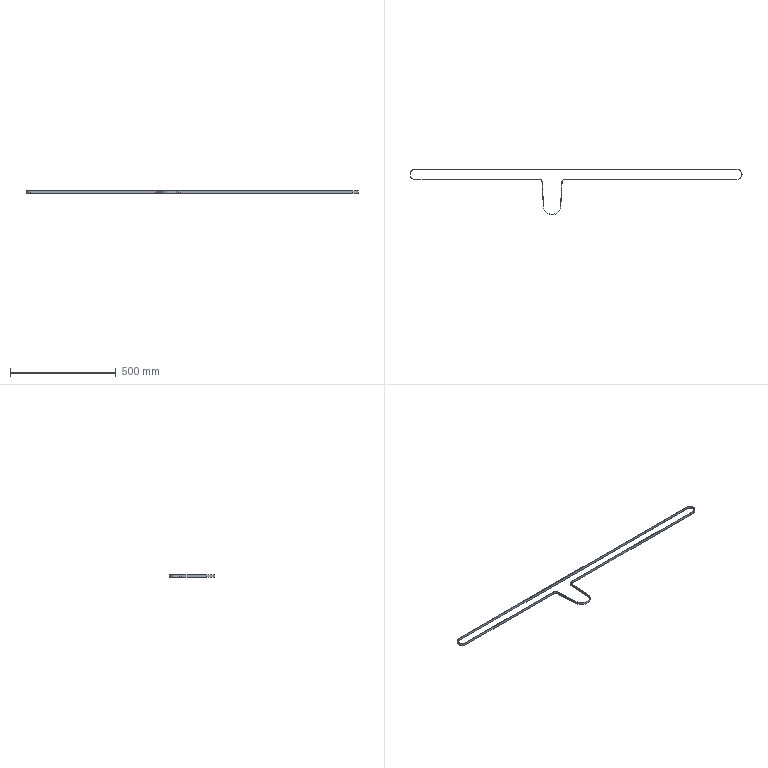Part | NX | features BREP 1 | 1 solid | 24 faces | box 1568 x 214.1 x 12 mm | volume 49856 mm3 | cylinder 12 | plane 12 | commonest cylinder face diameters 45 x3 47.4 x3 25 x2 27.4 x2 80 x1 82.4 x1
STEP:
#1=CARTESIAN_POINT('',(1415.214,8.857,-2.25));
#2=VERTEX_POINT('',#1);
#3=CARTESIAN_POINT('',(1392.714,31.357,-2.25));
#4=VERTEX_POINT('',#3);
#5=CARTESIAN_POINT('',(1392.714,8.857,-2.25));
#6=DIRECTION('',(0.,0.,1.));
#7=DIRECTION('',(-1.,0.,0.));
#8=AXIS2_PLACEMENT_3D('',#5,#6,#7);
#9=CIRCLE('',#8,22.5);
#10=EDGE_CURVE('',#2,#4,#9,.T.);
#11=ORIENTED_EDGE('',*,*,#10,.F.);
#12=CARTESIAN_POINT('',(1415.214,8.857,9.75));
#13=VERTEX_POINT('',#12);
#14=CARTESIAN_POINT('',(1415.214,8.857,-2.25));
#15=DIRECTION('',(0.,0.,1.));
#16=VECTOR('',#15,1000.);
#17=LINE('',#14,#16);
#18=EDGE_CURVE('',#2,#13,#17,.T.);
#19=ORIENTED_EDGE('',*,*,#18,.T.);
#20=CARTESIAN_POINT('',(1392.714,31.357,9.75));
#21=VERTEX_POINT('',#20);
#22=CARTESIAN_POINT('',(1392.714,8.857,9.75));
#23=DIRECTION('',(0.,0.,1.));
#24=DIRECTION('',(-1.,0.,0.));
#25=AXIS2_PLACEMENT_3D('',#22,#23,#24);
#26=CIRCLE('',#25,22.5);
#27=EDGE_CURVE('',#13,#21,#26,.T.);
#28=ORIENTED_EDGE('',*,*,#27,.T.);
#29=CARTESIAN_POINT('',(1392.714,31.357,-2.25));
#30=DIRECTION('',(0.,0.,1.));
#31=VECTOR('',#30,1000.);
#32=LINE('',#29,#31);
#33=EDGE_CURVE('',#4,#21,#32,.T.);
#34=ORIENTED_EDGE('',*,*,#33,.F.);
#35=EDGE_LOOP('',(#11,#19,#28,#34));
#36=FACE_BOUND('',#35,.T.);
#37=CARTESIAN_POINT('',(1392.714,8.857,-2.25));
#38=DIRECTION('',(0.,0.,1.));
#39=DIRECTION('',(1.,0.,0.));
#40=AXIS2_PLACEMENT_3D('',#37,#38,#39);
#41=CYLINDRICAL_SURFACE('',#40,22.5);
#42=ADVANCED_FACE('',(#36),#41,.F.);
#43=CARTESIAN_POINT('',(1392.714,-14.843,-2.25));
#44=VERTEX_POINT('',#43);
#45=CARTESIAN_POINT('',(1416.414,8.857,-2.25));
#46=VERTEX_POINT('',#45);
#47=CARTESIAN_POINT('',(1392.714,8.857,-2.25));
#48=DIRECTION('',(0.,0.,1.));
#49=DIRECTION('',(1.,0.,0.));
#50=AXIS2_PLACEMENT_3D('',#47,#48,#49);
#51=CIRCLE('',#50,23.7);
#52=EDGE_CURVE('',#44,#46,#51,.T.);
#53=ORIENTED_EDGE('',*,*,#52,.T.);
#54=CARTESIAN_POINT('',(1416.414,8.857,9.75));
#55=VERTEX_POINT('',#54);
#56=CARTESIAN_POINT('',(1416.414,8.857,-2.25));
#57=DIRECTION('',(0.,0.,1.));
#58=VECTOR('',#57,1000.);
#59=LINE('',#56,#58);
#60=EDGE_CURVE('',#46,#55,#59,.T.);
#61=ORIENTED_EDGE('',*,*,#60,.T.);
#62=CARTESIAN_POINT('',(1392.714,-14.843,9.75));
#63=VERTEX_POINT('',#62);
#64=CARTESIAN_POINT('',(1392.714,8.857,9.75));
#65=DIRECTION('',(0.,0.,1.));
#66=DIRECTION('',(1.,0.,0.));
#67=AXIS2_PLACEMENT_3D('',#64,#65,#66);
#68=CIRCLE('',#67,23.7);
#69=EDGE_CURVE('',#63,#55,#68,.T.);
#70=ORIENTED_EDGE('',*,*,#69,.F.);
#71=CARTESIAN_POINT('',(1392.714,-14.843,-2.25));
#72=DIRECTION('',(0.,0.,1.));
#73=VECTOR('',#72,1000.);
#74=LINE('',#71,#73);
#75=EDGE_CURVE('',#44,#63,#74,.T.);
#76=ORIENTED_EDGE('',*,*,#75,.F.);
#77=EDGE_LOOP('',(#53,#61,#70,#76));
#78=FACE_BOUND('',#77,.T.);
#79=CARTESIAN_POINT('',(1392.714,8.857,-2.25));
#80=DIRECTION('',(0.,0.,1.));
#81=DIRECTION('',(1.,0.,0.));
#82=AXIS2_PLACEMENT_3D('',#79,#80,#81);
#83=CYLINDRICAL_SURFACE('',#82,23.7);
#84=ADVANCED_FACE('',(#78),#83,.T.);
#85=ORIENTED_EDGE('',*,*,#60,.F.);
#86=CARTESIAN_POINT('',(1392.714,32.557,-2.25));
#87=VERTEX_POINT('',#86);
#88=CARTESIAN_POINT('',(1392.714,8.857,-2.25));
#89=DIRECTION('',(0.,0.,1.));
#90=DIRECTION('',(1.,0.,0.));
#91=AXIS2_PLACEMENT_3D('',#88,#89,#90);
#92=CIRCLE('',#91,23.7);
#93=EDGE_CURVE('',#46,#87,#92,.T.);
#94=ORIENTED_EDGE('',*,*,#93,.T.);
#95=CARTESIAN_POINT('',(1392.714,32.557,9.75));
#96=VERTEX_POINT('',#95);
#97=CARTESIAN_POINT('',(1392.714,32.557,-2.25));
#98=DIRECTION('',(0.,0.,1.));
#99=VECTOR('',#98,1000.);
#100=LINE('',#97,#99);
#101=EDGE_CURVE('',#87,#96,#100,.T.);
#102=ORIENTED_EDGE('',*,*,#101,.T.);
#103=CARTESIAN_POINT('',(1392.714,8.857,9.75));
#104=DIRECTION('',(0.,0.,1.));
#105=DIRECTION('',(1.,0.,0.));
#106=AXIS2_PLACEMENT_3D('',#103,#104,#105);
#107=CIRCLE('',#106,23.7);
#108=EDGE_CURVE('',#55,#96,#107,.T.);
#109=ORIENTED_EDGE('',*,*,#108,.F.);
#110=EDGE_LOOP('',(#85,#94,#102,#109));
#111=FACE_BOUND('',#110,.T.);
#112=CARTESIAN_POINT('',(1392.714,8.857,-2.25));
#113=DIRECTION('',(0.,0.,1.));
#114=DIRECTION('',(1.,0.,0.));
#115=AXIS2_PLACEMENT_3D('',#112,#113,#114);
#116=CYLINDRICAL_SURFACE('',#115,23.7);
#117=ADVANCED_FACE('',(#111),#116,.T.);
#118=CARTESIAN_POINT('',(579.214,-14.843,9.75));
#119=VERTEX_POINT('',#118);
#120=CARTESIAN_POINT('',(579.214,-14.843,9.75));
#121=DIRECTION('',(1.,0.,0.));
#122=VECTOR('',#121,1000.);
#123=LINE('',#120,#122);
#124=EDGE_CURVE('',#119,#63,#123,.T.);
#125=ORIENTED_EDGE('',*,*,#124,.F.);
#126=CARTESIAN_POINT('',(579.214,-14.843,-2.25));
#127=VERTEX_POINT('',#126);
#128=CARTESIAN_POINT('',(579.214,-14.843,-2.25));
#129=DIRECTION('',(0.,0.,1.));
#130=VECTOR('',#129,1000.);
#131=LINE('',#128,#130);
#132=EDGE_CURVE('',#127,#119,#131,.T.);
#133=ORIENTED_EDGE('',*,*,#132,.F.);
#134=CARTESIAN_POINT('',(579.214,-14.843,-2.25));
#135=DIRECTION('',(1.,0.,0.));
#136=VECTOR('',#135,1000.);
#137=LINE('',#134,#136);
#138=EDGE_CURVE('',#127,#44,#137,.T.);
#139=ORIENTED_EDGE('',*,*,#138,.T.);
#140=ORIENTED_EDGE('',*,*,#75,.T.);
#141=EDGE_LOOP('',(#125,#133,#139,#140));
#142=FACE_BOUND('',#141,.T.);
#143=CARTESIAN_POINT('',(579.214,-14.843,-2.25));
#144=DIRECTION('',(0.,-1.,0.));
#145=DIRECTION('',(0.,0.,-1.));
#146=AXIS2_PLACEMENT_3D('',#143,#144,#145);
#147=PLANE('',#146);
#148=ADVANCED_FACE('',(#142),#147,.T.);
#149=CARTESIAN_POINT('',(566.733,-26.656,9.75));
#150=VERTEX_POINT('',#149);
#151=CARTESIAN_POINT('',(579.214,-27.343,9.75));
#152=DIRECTION('',(0.,0.,-1.));
#153=DIRECTION('',(-1.,0.,0.));
#154=AXIS2_PLACEMENT_3D('',#151,#152,#153);
#155=CIRCLE('',#154,12.5);
#156=EDGE_CURVE('',#150,#119,#155,.T.);
#157=ORIENTED_EDGE('',*,*,#156,.F.);
#158=CARTESIAN_POINT('',(566.733,-26.656,-2.25));
#159=VERTEX_POINT('',#158);
#160=CARTESIAN_POINT('',(566.733,-26.656,-2.25));
#161=DIRECTION('',(0.,0.,1.));
#162=VECTOR('',#161,1000.);
#163=LINE('',#160,#162);
#164=EDGE_CURVE('',#159,#150,#163,.T.);
#165=ORIENTED_EDGE('',*,*,#164,.F.);
#166=CARTESIAN_POINT('',(579.214,-27.343,-2.25));
#167=DIRECTION('',(0.,0.,-1.));
#168=DIRECTION('',(-1.,0.,0.));
#169=AXIS2_PLACEMENT_3D('',#166,#167,#168);
#170=CIRCLE('',#169,12.5);
#171=EDGE_CURVE('',#159,#127,#170,.T.);
#172=ORIENTED_EDGE('',*,*,#171,.T.);
#173=ORIENTED_EDGE('',*,*,#132,.T.);
#174=EDGE_LOOP('',(#157,#165,#172,#173));
#175=FACE_BOUND('',#174,.T.);
#176=CARTESIAN_POINT('',(579.214,-27.343,-2.25));
#177=DIRECTION('',(0.,0.,1.));
#178=DIRECTION('',(1.,0.,0.));
#179=AXIS2_PLACEMENT_3D('',#176,#177,#178);
#180=CYLINDRICAL_SURFACE('',#179,12.5);
#181=ADVANCED_FACE('',(#175),#180,.F.);
#182=CARTESIAN_POINT('',(560.352,-142.607,9.75));
#183=VERTEX_POINT('',#182);
#184=CARTESIAN_POINT('',(560.352,-142.607,9.75));
#185=DIRECTION('',(0.05495,0.9985,0.));
#186=VECTOR('',#185,1000.);
#187=LINE('',#184,#186);
#188=EDGE_CURVE('',#183,#150,#187,.T.);
#189=ORIENTED_EDGE('',*,*,#188,.F.);
#190=CARTESIAN_POINT('',(560.352,-142.607,-2.25));
#191=VERTEX_POINT('',#190);
#192=CARTESIAN_POINT('',(560.352,-142.607,-2.25));
#193=DIRECTION('',(0.,0.,1.));
#194=VECTOR('',#193,1000.);
#195=LINE('',#192,#194);
#196=EDGE_CURVE('',#191,#183,#195,.T.);
#197=ORIENTED_EDGE('',*,*,#196,.F.);
#198=CARTESIAN_POINT('',(560.352,-142.607,-2.25));
#199=DIRECTION('',(0.05495,0.9985,0.));
#200=VECTOR('',#199,1000.);
#201=LINE('',#198,#200);
#202=EDGE_CURVE('',#191,#159,#201,.T.);
#203=ORIENTED_EDGE('',*,*,#202,.T.);
#204=ORIENTED_EDGE('',*,*,#164,.T.);
#205=EDGE_LOOP('',(#189,#197,#203,#204));
#206=FACE_BOUND('',#205,.T.);
#207=CARTESIAN_POINT('',(560.352,-142.607,-2.25));
#208=DIRECTION('',(0.9985,-0.05495,0.));
#209=DIRECTION('',(0.,0.,-1.));
#210=AXIS2_PLACEMENT_3D('',#207,#208,#209);
#211=PLANE('',#210);
#212=ADVANCED_FACE('',(#206),#211,.T.);
#213=CARTESIAN_POINT('',(478.077,-142.607,9.75));
#214=VERTEX_POINT('',#213);
#215=CARTESIAN_POINT('',(519.214,-140.343,9.75));
#216=DIRECTION('',(0.,0.,1.));
#217=DIRECTION('',(1.,0.,0.));
#218=AXIS2_PLACEMENT_3D('',#215,#216,#217);
#219=CIRCLE('',#218,41.2);
#220=EDGE_CURVE('',#214,#183,#219,.T.);
#221=ORIENTED_EDGE('',*,*,#220,.F.);
#222=CARTESIAN_POINT('',(478.077,-142.607,-2.25));
#223=VERTEX_POINT('',#222);
#224=CARTESIAN_POINT('',(478.077,-142.607,-2.25));
#225=DIRECTION('',(0.,0.,1.));
#226=VECTOR('',#225,1000.);
#227=LINE('',#224,#226);
#228=EDGE_CURVE('',#223,#214,#227,.T.);
#229=ORIENTED_EDGE('',*,*,#228,.F.);
#230=CARTESIAN_POINT('',(519.214,-140.343,-2.25));
#231=DIRECTION('',(0.,0.,1.));
#232=DIRECTION('',(1.,0.,0.));
#233=AXIS2_PLACEMENT_3D('',#230,#231,#232);
#234=CIRCLE('',#233,41.2);
#235=EDGE_CURVE('',#223,#191,#234,.T.);
#236=ORIENTED_EDGE('',*,*,#235,.T.);
#237=ORIENTED_EDGE('',*,*,#196,.T.);
#238=EDGE_LOOP('',(#221,#229,#236,#237));
#239=FACE_BOUND('',#238,.T.);
#240=CARTESIAN_POINT('',(519.214,-140.343,-2.25));
#241=DIRECTION('',(0.,0.,1.));
#242=DIRECTION('',(1.,0.,0.));
#243=AXIS2_PLACEMENT_3D('',#240,#241,#242);
#244=CYLINDRICAL_SURFACE('',#243,41.2);
#245=ADVANCED_FACE('',(#239),#244,.T.);
#246=CARTESIAN_POINT('',(471.695,-26.656,9.75));
#247=VERTEX_POINT('',#246);
#248=CARTESIAN_POINT('',(471.695,-26.656,9.75));
#249=DIRECTION('',(0.05495,-0.9985,0.));
#250=VECTOR('',#249,1000.);
#251=LINE('',#248,#250);
#252=EDGE_CURVE('',#247,#214,#251,.T.);
#253=ORIENTED_EDGE('',*,*,#252,.F.);
#254=CARTESIAN_POINT('',(471.695,-26.656,-2.25));
#255=VERTEX_POINT('',#254);
#256=CARTESIAN_POINT('',(471.695,-26.656,-2.25));
#257=DIRECTION('',(0.,0.,1.));
#258=VECTOR('',#257,1000.);
#259=LINE('',#256,#258);
#260=EDGE_CURVE('',#255,#247,#259,.T.);
#261=ORIENTED_EDGE('',*,*,#260,.F.);
#262=CARTESIAN_POINT('',(471.695,-26.656,-2.25));
#263=DIRECTION('',(0.05495,-0.9985,0.));
#264=VECTOR('',#263,1000.);
#265=LINE('',#262,#264);
#266=EDGE_CURVE('',#255,#223,#265,.T.);
#267=ORIENTED_EDGE('',*,*,#266,.T.);
#268=ORIENTED_EDGE('',*,*,#228,.T.);
#269=EDGE_LOOP('',(#253,#261,#267,#268));
#270=FACE_BOUND('',#269,.T.);
#271=CARTESIAN_POINT('',(471.695,-26.656,-2.25));
#272=DIRECTION('',(-0.9985,-0.05495,0.));
#273=DIRECTION('',(-0.05495,0.9985,0.));
#274=AXIS2_PLACEMENT_3D('',#271,#272,#273);
#275=PLANE('',#274);
#276=ADVANCED_FACE('',(#270),#275,.T.);
#277=CARTESIAN_POINT('',(459.214,-14.843,9.75));
#278=VERTEX_POINT('',#277);
#279=CARTESIAN_POINT('',(459.214,-27.343,9.75));
#280=DIRECTION('',(0.,0.,-1.));
#281=DIRECTION('',(-1.,0.,0.));
#282=AXIS2_PLACEMENT_3D('',#279,#280,#281);
#283=CIRCLE('',#282,12.5);
#284=EDGE_CURVE('',#278,#247,#283,.T.);
#285=ORIENTED_EDGE('',*,*,#284,.F.);
#286=CARTESIAN_POINT('',(459.214,-14.843,-2.25));
#287=VERTEX_POINT('',#286);
#288=CARTESIAN_POINT('',(459.214,-14.843,-2.25));
#289=DIRECTION('',(0.,0.,1.));
#290=VECTOR('',#289,1000.);
#291=LINE('',#288,#290);
#292=EDGE_CURVE('',#287,#278,#291,.T.);
#293=ORIENTED_EDGE('',*,*,#292,.F.);
#294=CARTESIAN_POINT('',(459.214,-27.343,-2.25));
#295=DIRECTION('',(0.,0.,-1.));
#296=DIRECTION('',(-1.,0.,0.));
#297=AXIS2_PLACEMENT_3D('',#294,#295,#296);
#298=CIRCLE('',#297,12.5);
#299=EDGE_CURVE('',#287,#255,#298,.T.);
#300=ORIENTED_EDGE('',*,*,#299,.T.);
#301=ORIENTED_EDGE('',*,*,#260,.T.);
#302=EDGE_LOOP('',(#285,#293,#300,#301));
#303=FACE_BOUND('',#302,.T.);
#304=CARTESIAN_POINT('',(459.214,-27.343,-2.25));
#305=DIRECTION('',(0.,0.,1.));
#306=DIRECTION('',(1.,0.,0.));
#307=AXIS2_PLACEMENT_3D('',#304,#305,#306);
#308=CYLINDRICAL_SURFACE('',#307,12.5);
#309=ADVANCED_FACE('',(#303),#308,.F.);
#310=CARTESIAN_POINT('',(-128.286,-14.843,9.75));
#311=VERTEX_POINT('',#310);
#312=CARTESIAN_POINT('',(-128.286,-14.843,9.75));
#313=DIRECTION('',(1.,0.,0.));
#314=VECTOR('',#313,1000.);
#315=LINE('',#312,#314);
#316=EDGE_CURVE('',#311,#278,#315,.T.);
#317=ORIENTED_EDGE('',*,*,#316,.F.);
#318=CARTESIAN_POINT('',(-128.286,-14.843,-2.25));
#319=VERTEX_POINT('',#318);
#320=CARTESIAN_POINT('',(-128.286,-14.843,-2.25));
#321=DIRECTION('',(0.,0.,1.));
#322=VECTOR('',#321,1000.);
#323=LINE('',#320,#322);
#324=EDGE_CURVE('',#319,#311,#323,.T.);
#325=ORIENTED_EDGE('',*,*,#324,.F.);
#326=CARTESIAN_POINT('',(-128.286,-14.843,-2.25));
#327=DIRECTION('',(1.,0.,0.));
#328=VECTOR('',#327,1000.);
#329=LINE('',#326,#328);
#330=EDGE_CURVE('',#319,#287,#329,.T.);
#331=ORIENTED_EDGE('',*,*,#330,.T.);
#332=ORIENTED_EDGE('',*,*,#292,.T.);
#333=EDGE_LOOP('',(#317,#325,#331,#332));
#334=FACE_BOUND('',#333,.T.);
#335=CARTESIAN_POINT('',(-128.286,-14.843,-2.25));
#336=DIRECTION('',(0.,-1.,0.));
#337=DIRECTION('',(-1.,0.,0.));
#338=AXIS2_PLACEMENT_3D('',#335,#336,#337);
#339=PLANE('',#338);
#340=ADVANCED_FACE('',(#334),#339,.T.);
#341=CARTESIAN_POINT('',(-128.286,32.557,9.75));
#342=VERTEX_POINT('',#341);
#343=CARTESIAN_POINT('',(-128.286,8.857,9.75));
#344=DIRECTION('',(0.,0.,1.));
#345=DIRECTION('',(1.,0.,0.));
#346=AXIS2_PLACEMENT_3D('',#343,#344,#345);
#347=CIRCLE('',#346,23.7);
#348=EDGE_CURVE('',#342,#311,#347,.T.);
#349=ORIENTED_EDGE('',*,*,#348,.F.);
#350=CARTESIAN_POINT('',(-128.286,32.557,-2.25));
#351=VERTEX_POINT('',#350);
#352=CARTESIAN_POINT('',(-128.286,32.557,-2.25));
#353=DIRECTION('',(0.,0.,1.));
#354=VECTOR('',#353,1000.);
#355=LINE('',#352,#354);
#356=EDGE_CURVE('',#351,#342,#355,.T.);
#357=ORIENTED_EDGE('',*,*,#356,.F.);
#358=CARTESIAN_POINT('',(-128.286,8.857,-2.25));
#359=DIRECTION('',(0.,0.,1.));
#360=DIRECTION('',(1.,0.,0.));
#361=AXIS2_PLACEMENT_3D('',#358,#359,#360);
#362=CIRCLE('',#361,23.7);
#363=EDGE_CURVE('',#351,#319,#362,.T.);
#364=ORIENTED_EDGE('',*,*,#363,.T.);
#365=ORIENTED_EDGE('',*,*,#324,.T.);
#366=EDGE_LOOP('',(#349,#357,#364,#365));
#367=FACE_BOUND('',#366,.T.);
#368=CARTESIAN_POINT('',(-128.286,8.857,-2.25));
#369=DIRECTION('',(0.,0.,1.));
#370=DIRECTION('',(1.,0.,0.));
#371=AXIS2_PLACEMENT_3D('',#368,#369,#370);
#372=CYLINDRICAL_SURFACE('',#371,23.7);
#373=ADVANCED_FACE('',(#367),#372,.T.);
#374=CARTESIAN_POINT('',(1392.714,32.557,9.75));
#375=DIRECTION('',(-1.,0.,0.));
#376=VECTOR('',#375,1000.);
#377=LINE('',#374,#376);
#378=EDGE_CURVE('',#96,#342,#377,.T.);
#379=ORIENTED_EDGE('',*,*,#378,.F.);
#380=ORIENTED_EDGE('',*,*,#101,.F.);
#381=CARTESIAN_POINT('',(1392.714,32.557,-2.25));
#382=DIRECTION('',(-1.,0.,0.));
#383=VECTOR('',#382,1000.);
#384=LINE('',#381,#383);
#385=EDGE_CURVE('',#87,#351,#384,.T.);
#386=ORIENTED_EDGE('',*,*,#385,.T.);
#387=ORIENTED_EDGE('',*,*,#356,.T.);
#388=EDGE_LOOP('',(#379,#380,#386,#387));
#389=FACE_BOUND('',#388,.T.);
#390=CARTESIAN_POINT('',(1392.714,32.557,-2.25));
#391=DIRECTION('',(0.,1.,0.));
#392=DIRECTION('',(1.,0.,0.));
#393=AXIS2_PLACEMENT_3D('',#390,#391,#392);
#394=PLANE('',#393);
#395=ADVANCED_FACE('',(#389),#394,.T.);
#396=ORIENTED_EDGE('',*,*,#52,.F.);
#397=ORIENTED_EDGE('',*,*,#138,.F.);
#398=ORIENTED_EDGE('',*,*,#171,.F.);
#399=ORIENTED_EDGE('',*,*,#202,.F.);
#400=ORIENTED_EDGE('',*,*,#235,.F.);
#401=ORIENTED_EDGE('',*,*,#266,.F.);
#402=ORIENTED_EDGE('',*,*,#299,.F.);
#403=ORIENTED_EDGE('',*,*,#330,.F.);
#404=ORIENTED_EDGE('',*,*,#363,.F.);
#405=ORIENTED_EDGE('',*,*,#385,.F.);
#406=ORIENTED_EDGE('',*,*,#93,.F.);
#407=EDGE_LOOP('',(#396,#397,#398,#399,#400,#401,#402,#403,#404,#405,#406));
#408=FACE_BOUND('',#407,.T.);
#409=CARTESIAN_POINT('',(472.894,-26.59,-2.25));
#410=VERTEX_POINT('',#409);
#411=CARTESIAN_POINT('',(479.275,-142.541,-2.25));
#412=VERTEX_POINT('',#411);
#413=CARTESIAN_POINT('',(479.275,-142.541,-2.25));
#414=DIRECTION('',(0.05495,-0.9985,0.));
#415=VECTOR('',#414,1000.);
#416=LINE('',#413,#415);
#417=EDGE_CURVE('',#410,#412,#416,.T.);
#418=ORIENTED_EDGE('',*,*,#417,.T.);
#419=CARTESIAN_POINT('',(559.154,-142.541,-2.25));
#420=VERTEX_POINT('',#419);
#421=CARTESIAN_POINT('',(519.214,-140.343,-2.25));
#422=DIRECTION('',(0.,0.,1.));
#423=DIRECTION('',(-1.,0.,0.));
#424=AXIS2_PLACEMENT_3D('',#421,#422,#423);
#425=CIRCLE('',#424,40.);
#426=EDGE_CURVE('',#412,#420,#425,.T.);
#427=ORIENTED_EDGE('',*,*,#426,.T.);
#428=CARTESIAN_POINT('',(565.535,-26.59,-2.25));
#429=VERTEX_POINT('',#428);
#430=CARTESIAN_POINT('',(565.535,-26.59,-2.25));
#431=DIRECTION('',(0.05495,0.9985,0.));
#432=VECTOR('',#431,1000.);
#433=LINE('',#430,#432);
#434=EDGE_CURVE('',#420,#429,#433,.T.);
#435=ORIENTED_EDGE('',*,*,#434,.T.);
#436=CARTESIAN_POINT('',(579.214,-13.643,-2.25));
#437=VERTEX_POINT('',#436);
#438=CARTESIAN_POINT('',(579.214,-27.343,-2.25));
#439=DIRECTION('',(0.,0.,-1.));
#440=DIRECTION('',(1.,0.,0.));
#441=AXIS2_PLACEMENT_3D('',#438,#439,#440);
#442=CIRCLE('',#441,13.7);
#443=EDGE_CURVE('',#429,#437,#442,.T.);
#444=ORIENTED_EDGE('',*,*,#443,.T.);
#445=CARTESIAN_POINT('',(1392.714,-13.643,-2.25));
#446=VERTEX_POINT('',#445);
#447=CARTESIAN_POINT('',(1392.714,-13.643,-2.25));
#448=DIRECTION('',(1.,0.,0.));
#449=VECTOR('',#448,1000.);
#450=LINE('',#447,#449);
#451=EDGE_CURVE('',#437,#446,#450,.T.);
#452=ORIENTED_EDGE('',*,*,#451,.T.);
#453=CARTESIAN_POINT('',(1392.714,8.857,-2.25));
#454=DIRECTION('',(0.,0.,1.));
#455=DIRECTION('',(-1.,0.,0.));
#456=AXIS2_PLACEMENT_3D('',#453,#454,#455);
#457=CIRCLE('',#456,22.5);
#458=EDGE_CURVE('',#446,#2,#457,.T.);
#459=ORIENTED_EDGE('',*,*,#458,.T.);
#460=ORIENTED_EDGE('',*,*,#10,.T.);
#461=CARTESIAN_POINT('',(-128.286,31.357,-2.25));
#462=VERTEX_POINT('',#461);
#463=CARTESIAN_POINT('',(-128.286,31.357,-2.25));
#464=DIRECTION('',(-1.,0.,0.));
#465=VECTOR('',#464,1000.);
#466=LINE('',#463,#465);
#467=EDGE_CURVE('',#4,#462,#466,.T.);
#468=ORIENTED_EDGE('',*,*,#467,.T.);
#469=CARTESIAN_POINT('',(-128.286,-13.643,-2.25));
#470=VERTEX_POINT('',#469);
#471=CARTESIAN_POINT('',(-128.286,8.857,-2.25));
#472=DIRECTION('',(0.,0.,1.));
#473=DIRECTION('',(-1.,0.,0.));
#474=AXIS2_PLACEMENT_3D('',#471,#472,#473);
#475=CIRCLE('',#474,22.5);
#476=EDGE_CURVE('',#462,#470,#475,.T.);
#477=ORIENTED_EDGE('',*,*,#476,.T.);
#478=CARTESIAN_POINT('',(459.214,-13.643,-2.25));
#479=VERTEX_POINT('',#478);
#480=CARTESIAN_POINT('',(459.214,-13.643,-2.25));
#481=DIRECTION('',(1.,0.,0.));
#482=VECTOR('',#481,1000.);
#483=LINE('',#480,#482);
#484=EDGE_CURVE('',#470,#479,#483,.T.);
#485=ORIENTED_EDGE('',*,*,#484,.T.);
#486=CARTESIAN_POINT('',(459.214,-27.343,-2.25));
#487=DIRECTION('',(0.,0.,-1.));
#488=DIRECTION('',(1.,0.,0.));
#489=AXIS2_PLACEMENT_3D('',#486,#487,#488);
#490=CIRCLE('',#489,13.7);
#491=EDGE_CURVE('',#479,#410,#490,.T.);
#492=ORIENTED_EDGE('',*,*,#491,.T.);
#493=EDGE_LOOP('',(#418,#427,#435,#444,#452,#459,#460,#468,#477,#485,#492));
#494=FACE_BOUND('',#493,.T.);
#495=CARTESIAN_POINT('',(1392.714,8.857,-2.25));
#496=DIRECTION('',(0.,0.,1.));
#497=DIRECTION('',(1.,0.,0.));
#498=AXIS2_PLACEMENT_3D('',#495,#496,#497);
#499=PLANE('',#498);
#500=ADVANCED_FACE('',(#408,#494),#499,.F.);
#501=ORIENTED_EDGE('',*,*,#69,.T.);
#502=ORIENTED_EDGE('',*,*,#108,.T.);
#503=ORIENTED_EDGE('',*,*,#378,.T.);
#504=ORIENTED_EDGE('',*,*,#348,.T.);
#505=ORIENTED_EDGE('',*,*,#316,.T.);
#506=ORIENTED_EDGE('',*,*,#284,.T.);
#507=ORIENTED_EDGE('',*,*,#252,.T.);
#508=ORIENTED_EDGE('',*,*,#220,.T.);
#509=ORIENTED_EDGE('',*,*,#188,.T.);
#510=ORIENTED_EDGE('',*,*,#156,.T.);
#511=ORIENTED_EDGE('',*,*,#124,.T.);
#512=EDGE_LOOP('',(#501,#502,#503,#504,#505,#506,#507,#508,#509,#510,#511));
#513=FACE_BOUND('',#512,.T.);
#514=CARTESIAN_POINT('',(479.275,-142.541,9.75));
#515=VERTEX_POINT('',#514);
#516=CARTESIAN_POINT('',(559.154,-142.541,9.75));
#517=VERTEX_POINT('',#516);
#518=CARTESIAN_POINT('',(519.214,-140.343,9.75));
#519=DIRECTION('',(0.,0.,1.));
#520=DIRECTION('',(-1.,0.,0.));
#521=AXIS2_PLACEMENT_3D('',#518,#519,#520);
#522=CIRCLE('',#521,40.);
#523=EDGE_CURVE('',#515,#517,#522,.T.);
#524=ORIENTED_EDGE('',*,*,#523,.F.);
#525=CARTESIAN_POINT('',(472.894,-26.59,9.75));
#526=VERTEX_POINT('',#525);
#527=CARTESIAN_POINT('',(479.275,-142.541,9.75));
#528=DIRECTION('',(0.05495,-0.9985,0.));
#529=VECTOR('',#528,1000.);
#530=LINE('',#527,#529);
#531=EDGE_CURVE('',#526,#515,#530,.T.);
#532=ORIENTED_EDGE('',*,*,#531,.F.);
#533=CARTESIAN_POINT('',(459.214,-13.643,9.75));
#534=VERTEX_POINT('',#533);
#535=CARTESIAN_POINT('',(459.214,-27.343,9.75));
#536=DIRECTION('',(0.,0.,-1.));
#537=DIRECTION('',(1.,0.,0.));
#538=AXIS2_PLACEMENT_3D('',#535,#536,#537);
#539=CIRCLE('',#538,13.7);
#540=EDGE_CURVE('',#534,#526,#539,.T.);
#541=ORIENTED_EDGE('',*,*,#540,.F.);
#542=CARTESIAN_POINT('',(-128.286,-13.643,9.75));
#543=VERTEX_POINT('',#542);
#544=CARTESIAN_POINT('',(459.214,-13.643,9.75));
#545=DIRECTION('',(1.,0.,0.));
#546=VECTOR('',#545,1000.);
#547=LINE('',#544,#546);
#548=EDGE_CURVE('',#543,#534,#547,.T.);
#549=ORIENTED_EDGE('',*,*,#548,.F.);
#550=CARTESIAN_POINT('',(-128.286,31.357,9.75));
#551=VERTEX_POINT('',#550);
#552=CARTESIAN_POINT('',(-128.286,8.857,9.75));
#553=DIRECTION('',(0.,0.,1.));
#554=DIRECTION('',(-1.,0.,0.));
#555=AXIS2_PLACEMENT_3D('',#552,#553,#554);
#556=CIRCLE('',#555,22.5);
#557=EDGE_CURVE('',#551,#543,#556,.T.);
#558=ORIENTED_EDGE('',*,*,#557,.F.);
#559=CARTESIAN_POINT('',(-128.286,31.357,9.75));
#560=DIRECTION('',(-1.,0.,0.));
#561=VECTOR('',#560,1000.);
#562=LINE('',#559,#561);
#563=EDGE_CURVE('',#21,#551,#562,.T.);
#564=ORIENTED_EDGE('',*,*,#563,.F.);
#565=ORIENTED_EDGE('',*,*,#27,.F.);
#566=CARTESIAN_POINT('',(1392.714,-13.643,9.75));
#567=VERTEX_POINT('',#566);
#568=CARTESIAN_POINT('',(1392.714,8.857,9.75));
#569=DIRECTION('',(0.,0.,1.));
#570=DIRECTION('',(-1.,0.,0.));
#571=AXIS2_PLACEMENT_3D('',#568,#569,#570);
#572=CIRCLE('',#571,22.5);
#573=EDGE_CURVE('',#567,#13,#572,.T.);
#574=ORIENTED_EDGE('',*,*,#573,.F.);
#575=CARTESIAN_POINT('',(579.214,-13.643,9.75));
#576=VERTEX_POINT('',#575);
#577=CARTESIAN_POINT('',(1392.714,-13.643,9.75));
#578=DIRECTION('',(1.,0.,0.));
#579=VECTOR('',#578,1000.);
#580=LINE('',#577,#579);
#581=EDGE_CURVE('',#576,#567,#580,.T.);
#582=ORIENTED_EDGE('',*,*,#581,.F.);
#583=CARTESIAN_POINT('',(565.535,-26.59,9.75));
#584=VERTEX_POINT('',#583);
#585=CARTESIAN_POINT('',(579.214,-27.343,9.75));
#586=DIRECTION('',(0.,0.,-1.));
#587=DIRECTION('',(1.,0.,0.));
#588=AXIS2_PLACEMENT_3D('',#585,#586,#587);
#589=CIRCLE('',#588,13.7);
#590=EDGE_CURVE('',#584,#576,#589,.T.);
#591=ORIENTED_EDGE('',*,*,#590,.F.);
#592=CARTESIAN_POINT('',(565.535,-26.59,9.75));
#593=DIRECTION('',(0.05495,0.9985,0.));
#594=VECTOR('',#593,1000.);
#595=LINE('',#592,#594);
#596=EDGE_CURVE('',#517,#584,#595,.T.);
#597=ORIENTED_EDGE('',*,*,#596,.F.);
#598=EDGE_LOOP('',(#524,#532,#541,#549,#558,#564,#565,#574,#582,#591,#597));
#599=FACE_BOUND('',#598,.T.);
#600=CARTESIAN_POINT('',(1392.714,8.857,9.75));
#601=DIRECTION('',(0.,0.,1.));
#602=DIRECTION('',(1.,0.,0.));
#603=AXIS2_PLACEMENT_3D('',#600,#601,#602);
#604=PLANE('',#603);
#605=ADVANCED_FACE('',(#513,#599),#604,.T.);
#606=ORIENTED_EDGE('',*,*,#523,.T.);
#607=CARTESIAN_POINT('',(559.154,-142.541,-2.25));
#608=DIRECTION('',(0.,0.,1.));
#609=VECTOR('',#608,1000.);
#610=LINE('',#607,#609);
#611=EDGE_CURVE('',#420,#517,#610,.T.);
#612=ORIENTED_EDGE('',*,*,#611,.F.);
#613=ORIENTED_EDGE('',*,*,#426,.F.);
#614=CARTESIAN_POINT('',(479.275,-142.541,-2.25));
#615=DIRECTION('',(0.,0.,1.));
#616=VECTOR('',#615,1000.);
#617=LINE('',#614,#616);
#618=EDGE_CURVE('',#412,#515,#617,.T.);
#619=ORIENTED_EDGE('',*,*,#618,.T.);
#620=EDGE_LOOP('',(#606,#612,#613,#619));
#621=FACE_BOUND('',#620,.T.);
#622=CARTESIAN_POINT('',(519.214,-140.343,-2.25));
#623=DIRECTION('',(0.,0.,1.));
#624=DIRECTION('',(1.,0.,0.));
#625=AXIS2_PLACEMENT_3D('',#622,#623,#624);
#626=CYLINDRICAL_SURFACE('',#625,40.);
#627=ADVANCED_FACE('',(#621),#626,.F.);
#628=ORIENTED_EDGE('',*,*,#531,.T.);
#629=ORIENTED_EDGE('',*,*,#618,.F.);
#630=ORIENTED_EDGE('',*,*,#417,.F.);
#631=CARTESIAN_POINT('',(472.894,-26.59,-2.25));
#632=DIRECTION('',(0.,0.,1.));
#633=VECTOR('',#632,1000.);
#634=LINE('',#631,#633);
#635=EDGE_CURVE('',#410,#526,#634,.T.);
#636=ORIENTED_EDGE('',*,*,#635,.T.);
#637=EDGE_LOOP('',(#628,#629,#630,#636));
#638=FACE_BOUND('',#637,.T.);
#639=CARTESIAN_POINT('',(479.275,-142.541,-2.25));
#640=DIRECTION('',(-0.9985,-0.05495,0.));
#641=DIRECTION('',(-0.05495,0.9985,0.));
#642=AXIS2_PLACEMENT_3D('',#639,#640,#641);
#643=PLANE('',#642);
#644=ADVANCED_FACE('',(#638),#643,.F.);
#645=ORIENTED_EDGE('',*,*,#540,.T.);
#646=ORIENTED_EDGE('',*,*,#635,.F.);
#647=ORIENTED_EDGE('',*,*,#491,.F.);
#648=CARTESIAN_POINT('',(459.214,-13.643,-2.25));
#649=DIRECTION('',(0.,0.,1.));
#650=VECTOR('',#649,1000.);
#651=LINE('',#648,#650);
#652=EDGE_CURVE('',#479,#534,#651,.T.);
#653=ORIENTED_EDGE('',*,*,#652,.T.);
#654=EDGE_LOOP('',(#645,#646,#647,#653));
#655=FACE_BOUND('',#654,.T.);
#656=CARTESIAN_POINT('',(459.214,-27.343,-2.25));
#657=DIRECTION('',(0.,0.,1.));
#658=DIRECTION('',(1.,0.,0.));
#659=AXIS2_PLACEMENT_3D('',#656,#657,#658);
#660=CYLINDRICAL_SURFACE('',#659,13.7);
#661=ADVANCED_FACE('',(#655),#660,.T.);
#662=ORIENTED_EDGE('',*,*,#548,.T.);
#663=ORIENTED_EDGE('',*,*,#652,.F.);
#664=ORIENTED_EDGE('',*,*,#484,.F.);
#665=CARTESIAN_POINT('',(-128.286,-13.643,-2.25));
#666=DIRECTION('',(0.,0.,1.));
#667=VECTOR('',#666,1000.);
#668=LINE('',#665,#667);
#669=EDGE_CURVE('',#470,#543,#668,.T.);
#670=ORIENTED_EDGE('',*,*,#669,.T.);
#671=EDGE_LOOP('',(#662,#663,#664,#670));
#672=FACE_BOUND('',#671,.T.);
#673=CARTESIAN_POINT('',(459.214,-13.643,-2.25));
#674=DIRECTION('',(0.,-1.,0.));
#675=DIRECTION('',(0.,0.,-1.));
#676=AXIS2_PLACEMENT_3D('',#673,#674,#675);
#677=PLANE('',#676);
#678=ADVANCED_FACE('',(#672),#677,.F.);
#679=ORIENTED_EDGE('',*,*,#557,.T.);
#680=ORIENTED_EDGE('',*,*,#669,.F.);
#681=ORIENTED_EDGE('',*,*,#476,.F.);
#682=CARTESIAN_POINT('',(-128.286,31.357,-2.25));
#683=DIRECTION('',(0.,0.,1.));
#684=VECTOR('',#683,1000.);
#685=LINE('',#682,#684);
#686=EDGE_CURVE('',#462,#551,#685,.T.);
#687=ORIENTED_EDGE('',*,*,#686,.T.);
#688=EDGE_LOOP('',(#679,#680,#681,#687));
#689=FACE_BOUND('',#688,.T.);
#690=CARTESIAN_POINT('',(-128.286,8.857,-2.25));
#691=DIRECTION('',(0.,0.,1.));
#692=DIRECTION('',(1.,0.,0.));
#693=AXIS2_PLACEMENT_3D('',#690,#691,#692);
#694=CYLINDRICAL_SURFACE('',#693,22.5);
#695=ADVANCED_FACE('',(#689),#694,.F.);
#696=ORIENTED_EDGE('',*,*,#563,.T.);
#697=ORIENTED_EDGE('',*,*,#686,.F.);
#698=ORIENTED_EDGE('',*,*,#467,.F.);
#699=ORIENTED_EDGE('',*,*,#33,.T.);
#700=EDGE_LOOP('',(#696,#697,#698,#699));
#701=FACE_BOUND('',#700,.T.);
#702=CARTESIAN_POINT('',(-128.286,31.357,-2.25));
#703=DIRECTION('',(0.,1.,0.));
#704=DIRECTION('',(1.,0.,0.));
#705=AXIS2_PLACEMENT_3D('',#702,#703,#704);
#706=PLANE('',#705);
#707=ADVANCED_FACE('',(#701),#706,.F.);
#708=ORIENTED_EDGE('',*,*,#18,.F.);
#709=ORIENTED_EDGE('',*,*,#458,.F.);
#710=CARTESIAN_POINT('',(1392.714,-13.643,-2.25));
#711=DIRECTION('',(0.,0.,1.));
#712=VECTOR('',#711,1000.);
#713=LINE('',#710,#712);
#714=EDGE_CURVE('',#446,#567,#713,.T.);
#715=ORIENTED_EDGE('',*,*,#714,.T.);
#716=ORIENTED_EDGE('',*,*,#573,.T.);
#717=EDGE_LOOP('',(#708,#709,#715,#716));
#718=FACE_BOUND('',#717,.T.);
#719=CARTESIAN_POINT('',(1392.714,8.857,-2.25));
#720=DIRECTION('',(0.,0.,1.));
#721=DIRECTION('',(1.,0.,0.));
#722=AXIS2_PLACEMENT_3D('',#719,#720,#721);
#723=CYLINDRICAL_SURFACE('',#722,22.5);
#724=ADVANCED_FACE('',(#718),#723,.F.);
#725=ORIENTED_EDGE('',*,*,#581,.T.);
#726=ORIENTED_EDGE('',*,*,#714,.F.);
#727=ORIENTED_EDGE('',*,*,#451,.F.);
#728=CARTESIAN_POINT('',(579.214,-13.643,-2.25));
#729=DIRECTION('',(0.,0.,1.));
#730=VECTOR('',#729,1000.);
#731=LINE('',#728,#730);
#732=EDGE_CURVE('',#437,#576,#731,.T.);
#733=ORIENTED_EDGE('',*,*,#732,.T.);
#734=EDGE_LOOP('',(#725,#726,#727,#733));
#735=FACE_BOUND('',#734,.T.);
#736=CARTESIAN_POINT('',(1392.714,-13.643,-2.25));
#737=DIRECTION('',(0.,-1.,0.));
#738=DIRECTION('',(0.,0.,-1.));
#739=AXIS2_PLACEMENT_3D('',#736,#737,#738);
#740=PLANE('',#739);
#741=ADVANCED_FACE('',(#735),#740,.F.);
#742=ORIENTED_EDGE('',*,*,#590,.T.);
#743=ORIENTED_EDGE('',*,*,#732,.F.);
#744=ORIENTED_EDGE('',*,*,#443,.F.);
#745=CARTESIAN_POINT('',(565.535,-26.59,-2.25));
#746=DIRECTION('',(0.,0.,1.));
#747=VECTOR('',#746,1000.);
#748=LINE('',#745,#747);
#749=EDGE_CURVE('',#429,#584,#748,.T.);
#750=ORIENTED_EDGE('',*,*,#749,.T.);
#751=EDGE_LOOP('',(#742,#743,#744,#750));
#752=FACE_BOUND('',#751,.T.);
#753=CARTESIAN_POINT('',(579.214,-27.343,-2.25));
#754=DIRECTION('',(0.,0.,1.));
#755=DIRECTION('',(1.,0.,0.));
#756=AXIS2_PLACEMENT_3D('',#753,#754,#755);
#757=CYLINDRICAL_SURFACE('',#756,13.7);
#758=ADVANCED_FACE('',(#752),#757,.T.);
#759=ORIENTED_EDGE('',*,*,#596,.T.);
#760=ORIENTED_EDGE('',*,*,#749,.F.);
#761=ORIENTED_EDGE('',*,*,#434,.F.);
#762=ORIENTED_EDGE('',*,*,#611,.T.);
#763=EDGE_LOOP('',(#759,#760,#761,#762));
#764=FACE_BOUND('',#763,.T.);
#765=CARTESIAN_POINT('',(565.535,-26.59,-2.25));
#766=DIRECTION('',(0.9985,-0.05495,0.));
#767=DIRECTION('',(0.,0.,-1.));
#768=AXIS2_PLACEMENT_3D('',#765,#766,#767);
#769=PLANE('',#768);
#770=ADVANCED_FACE('',(#764),#769,.F.);
#771=CLOSED_SHELL('',(#42,#84,#117,#148,#181,#212,#245,#276,#309,#340,#373,#395,#500,#605,#627,#644,#661,#678,#695,#707,#724,#741,#758,#770));
#772=MANIFOLD_SOLID_BREP('',#771);
#773=(LENGTH_UNIT()NAMED_UNIT(*)SI_UNIT(.MILLI.,.METRE.));
#774=UNCERTAINTY_MEASURE_WITH_UNIT(LENGTH_MEASURE(0.00001),#773,'','');
#775=(NAMED_UNIT(*)PLANE_ANGLE_UNIT()SI_UNIT($,.RADIAN.));
#776=(NAMED_UNIT(*)SI_UNIT($,.STERADIAN.)SOLID_ANGLE_UNIT());
#777=(GEOMETRIC_REPRESENTATION_CONTEXT(3)GLOBAL_UNCERTAINTY_ASSIGNED_CONTEXT((#774))GLOBAL_UNIT_ASSIGNED_CONTEXT((#773,#775,#776))REPRESENTATION_CONTEXT('',''));
#778=ADVANCED_BREP_SHAPE_REPRESENTATION('',(#772),#777);